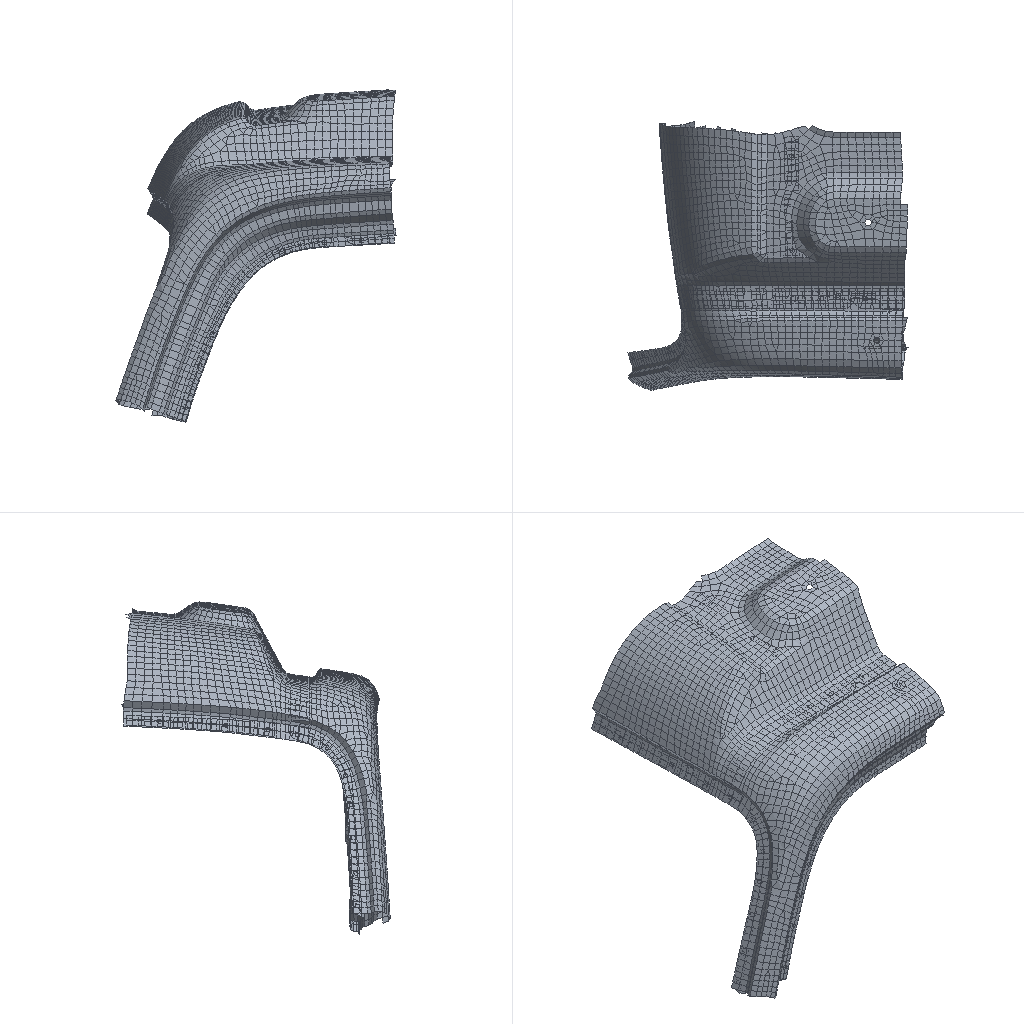Simulation study | nastran
Set-up summary:
category,name,step,type,value,unit,region
solver,nx_nastran
units,not stated in the deck,,not stated
analysis,deck,,static,static
analysis,solution,,SOL,101
load_step,SUBCASE 2,2,SUBCASE,SPC=2 LOAD=3
load_step,SUBCASE 3,3,SUBCASE,SPC=2 LOAD=4
load_step,SUBCASE 4,4,SUBCASE,SPC=2 LOAD=5
load_step,requested,,,3
mesh,nodes,,,5312
mesh,elements,,,4792
element_type,CHEXA,,unverified,32
element_type,CQUAD4,,shell,4543
element_type,CTRIA3,,shell,249
load,load commands in deck,,count,3
bc,support commands in deck,,count,233
check,setup vs results,,match,"every grid point's frame and coordinates and every element id; grid points of CHEXA, CQUAD4, CTRIA3 elements"
Nastran input file, long lists of numbers shortened:
$$------------------------------------------------------------------------------$
$$                                                                              $
$$ NASTRAN Input Deck Generated by HyperMesh Version  :10.0buil                 $
$$ Generated using HyperMesh-Nastran Template Version : 10.0build60
$$                                                                              $
$$   Template:  general                                                         $
$$                                                                              $
$$------------------------------------------------------------------------------$
$$------------------------------------------------------------------------------$
$$                      Executive Control Cards                                 $
$$------------------------------------------------------------------------------$
SOL 101
CEND
$$------------------------------------------------------------------------------$
$$                      Case Control Cards                                      $
$$------------------------------------------------------------------------------$
  DISPLACEMENT = ALL
  ESE = ALL
$
$HMNAME LOADSTEP               2"fx"
SUBCASE       2
  LABEL=    fx
  SPC =        2
  LOAD =        3
$
$HMNAME LOADSTEP               3"fy"
SUBCASE       3
  LABEL=    fy
  SPC =        2
  LOAD =        4
$
$HMNAME LOADSTEP               4"fz"
SUBCASE       4
  LABEL=    fz
  SPC =        2
  LOAD =        5
$$------------------------------------------------------------------------------$
$$                      Bulk Data Cards                                         $
$$------------------------------------------------------------------------------$
BEGIN BULK
PARAM,POST,-1
$$
$$  GRID Data
$$
GRID          45        -598.898-842.1481708.803
GRID          46        -593.222-832.0261710.596
$ (5310 more lines like these left out)
$$
$$  SPOINT Data
$$
$$
$$------------------------------------------------------------------------------$
$$             Group Definitions                                                $
$$------------------------------------------------------------------------------$
$$
$$ RBE2 Elements - Multiple dependent nodes
$$
RBE2     101480284099624  123456  619294  619295  619324  619325  619410+
+         619411  619452  619481  621803  621804  621837  621870  621871+
+         621910  621911  622313  622314  622315  622361  622362  622363+
+         622394  622395  623176  623177  623216  623217  623261  623262+
+         631183  631184  631808  631809  633660  640248  640249  640254+
+         640255  641185  641186  641196  641197  641997  641998  641999+
+         642003  642004  642005  642821  643142  643147  643154  643229+
+         643230  643243  643244  648117  648118  648181  648228  648257+
+         648258  648273  648274  649193  649194  649195  649196 3748698+
+        3748705 3748706 3748909 3748910 3750076 3750077 3750157 3750158+
+        3750211 3750212 3750258 3755181 3755185 3755186 3755187
$
$HMMOVE 57005014
$        1014802
$
$
$  RBE3 Elements
$
RBE3      327939         3757097  1234560.020327     123 37483320.717797+
+            123 37483330.254664     123 37483290.007212     123 3748330
RBE3      327940         3757098  1234560.529623     123 37483320.169946+
+            123 37483330.072984     123 37483290.227448     123 3748330
$ (508 more lines like these left out)
$
$HMMOVE 57005012
$         327939THRU      327942  327944THRU      327951  327953THRU      327956
$         328425THRU      328428  328430THRU      328437  328439THRU      328442
$         328461THRU      328464  328466THRU      328473  328475THRU      328478
$         332007THRU      332010  332012THRU      332015  332277THRU      332280
$         332282THRU      332289  332291THRU      332298  332300THRU      332303
$         340341THRU      340344  340346THRU      340353  340355THRU      340362
$         340364THRU      340371  340373THRU      340380  340382THRU      340389
$         340391THRU      340394  340512THRU      340515  340517THRU      340520
$         340539THRU      340542  340544THRU      340551  340553THRU      340560
$         340562THRU      340565  340575THRU      340578  340580THRU      340583
$         340593THRU      340596  340598THRU      340601  345867THRU      345870
$         345872THRU      345879  345881THRU      345888  345890THRU      345897
$         345899THRU      345906  345908THRU      345915  345917THRU      345924
$         345926THRU      345933  345935THRU      345942  345944THRU      345951
$         345953THRU      345956
$
$$
$$  CTRIA3 Data
$$
CTRIA3    250881       1  619277  619278  619341
CTRIA3    250915       1  622487  622486  622417
$ (247 more lines like these left out)
$
$HMMOVE 54001010
$         250881  250915THRU      250924  250926THRU      250931  250986  251140
$       THRU      251142  251166THRU      251167  251180  251192  251198  251291
$ (47 more lines like these left out)
CQUAD4    251500       1  615735  615726  615727  615734
CQUAD4    251501       1  615726  615735  615730  615725
$ (4541 more lines like these left out)
$
$HMMOVE 54001010
$         251500THRU      251505  253693THRU      253702  253750THRU      253755
$         253780THRU      253793  253846THRU      253862  253883THRU      253925
$ (208 more lines like these left out)
CHEXA     327943      10 3757097 3757100 3757099 3757098 3757101 3757104+
+        3757103 3757102
CHEXA     327952      10 3757106 3757109 3757108 3757107 3757110 3757113+
+        3757112 3757111
$ (60 more lines like these left out)
$
$HMMOVE 57005011
$         327943  327952  328429  328438  328465  328474  332011  332281  332290
$         332299  340345  340354  340363  340372  340381  340390  340516  340543
$ (56 more lines like these left out)
PSHELL         1       10.8            1               1
$
$HMNAME PROP                   2"120" 4
$HWCOLOR PROP                  2       3
PSHELL         2       11.2            1               1
$$
$$  PSOLID Data
$
$HMNAME PROP                  10"spot" 5
$HWCOLOR PROP                 10       3
PSOLID        10       1
$$
$$------------------------------------------------------------------------------$
$$                      Material Definition Cards                               $
$$------------------------------------------------------------------------------$
$$--------------------------------------------------------------
$$ HYPERMESH TAGS
$$--------------------------------------------------------------
$$BEGIN TAGS
$$END TAGS
$$
$$  MAT1 Data
$
$HMNAME MAT                    1"steel" "MAT1"
$HWCOLOR MAT                   1       3
MAT1           1210000.0        0.3     7.80E-09
$$
$$
$$
$$------------------------------------------------------------------------------$
$ (42 more lines like these left out)
SPC            2     400  1234560.0
SPC            2     388  1234560.0
SPC            2     262  1234560.0
SPC            2 3750051  1234560.0
$ (229 more lines like these left out)
$$
$$  FORCE Data
$$
FORCE          384099624       01.0     140.0   0.0     0.0
FORCE          484099624       01.0     0.0     320.0   0.0
FORCE          584099624       01.0     0.0     0.0     140.0
$HMASSEM 5700100       5 5700100
$HMASSEM_IDS    5700101057002010
$HMASSEM 5400200       6 sidebody_R
$HMASSEM_IDS    570050115700501257005014
$HMASSEM 5400100       7 sidebody_L
$HMASSEM_IDS    54001010540070105400103054003010
$HMASSEM 5700101       3 N211
$HMASSEM_ASSEM_ID        5700100 5400200 5400100
$
ENDDATA
Results summary:
result,analysis,,,static
result,last_loadstep,,,3
result,primary field,,,displacements
result,max displacement,,,1.797,model units